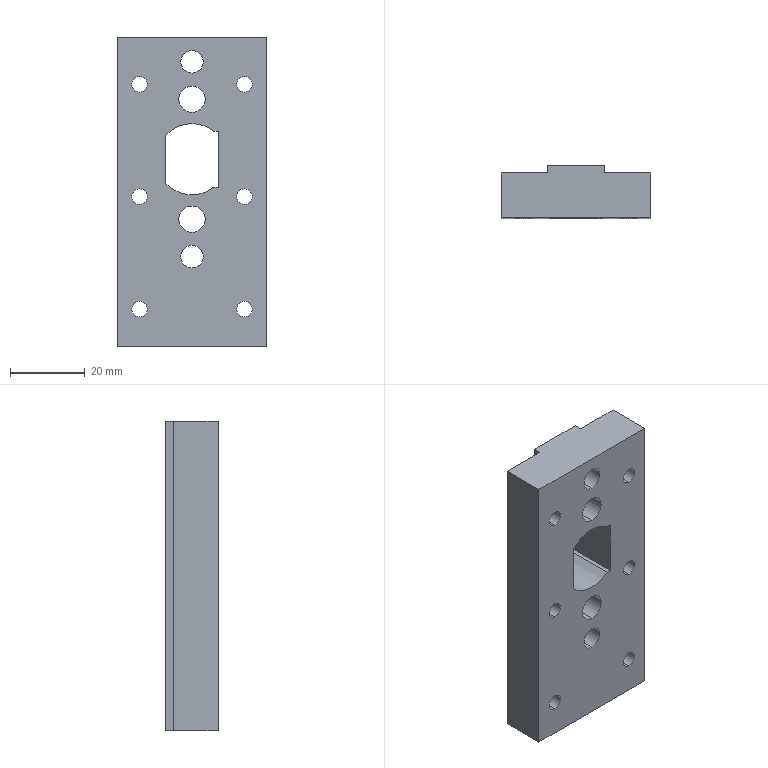Part | STEP file | secondary slingshot input track | 1 solid | 43 faces | box 40 x 14 x 82.5 mm | volume 35227 mm3 | cylinder 27 | plane 16 | commonest cylinder face diameters 4.2 x12 6 x4 7 x4 11 x4 19 x3